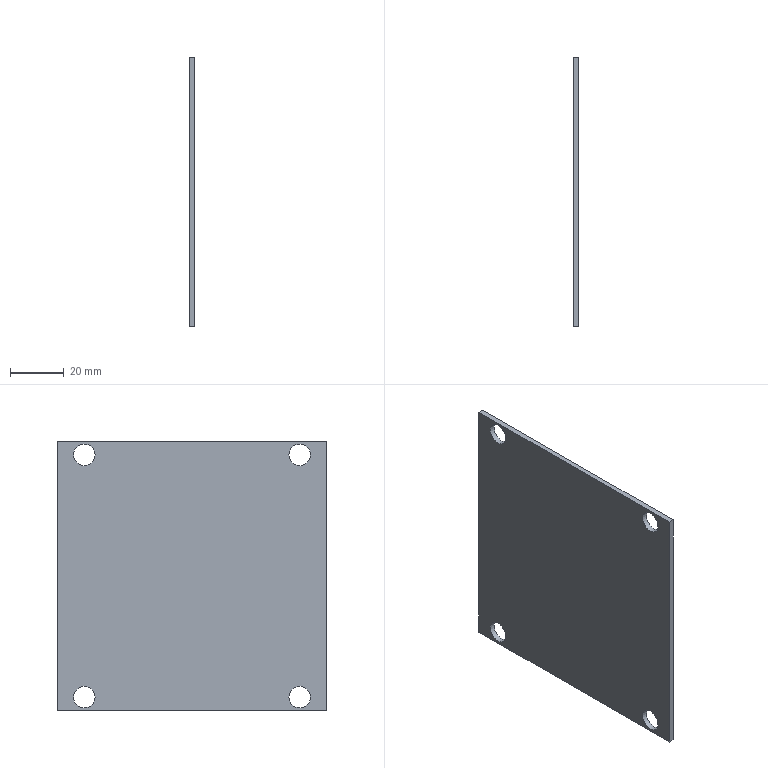Part | NX | features solid 2 | 1 solid | 10 faces | box 2 x 100 x 100 mm | volume 19598 mm3 | plane 6 | cylinder 4 | commonest cylinder face diameters 8 x4
STEP:
#1=CARTESIAN_POINT('',(1107.,-206.,-480.));
#2=VERTEX_POINT('',#1);
#3=CARTESIAN_POINT('',(1109.,-206.,-480.));
#4=VERTEX_POINT('',#3);
#5=CARTESIAN_POINT('',(1107.,-206.,-480.));
#6=DIRECTION('',(1.,0.,0.));
#7=VECTOR('',#6,1000.);
#8=LINE('',#5,#7);
#9=EDGE_CURVE('',#2,#4,#8,.T.);
#10=ORIENTED_EDGE('',*,*,#9,.F.);
#11=CARTESIAN_POINT('',(1107.,-106.,-480.));
#12=VERTEX_POINT('',#11);
#13=CARTESIAN_POINT('',(1107.,-106.,-480.));
#14=DIRECTION('',(0.,-1.,0.));
#15=VECTOR('',#14,1000.);
#16=LINE('',#13,#15);
#17=EDGE_CURVE('',#12,#2,#16,.T.);
#18=ORIENTED_EDGE('',*,*,#17,.F.);
#19=CARTESIAN_POINT('',(1109.,-106.,-480.));
#20=VERTEX_POINT('',#19);
#21=CARTESIAN_POINT('',(1107.,-106.,-480.));
#22=DIRECTION('',(1.,0.,0.));
#23=VECTOR('',#22,1000.);
#24=LINE('',#21,#23);
#25=EDGE_CURVE('',#12,#20,#24,.T.);
#26=ORIENTED_EDGE('',*,*,#25,.T.);
#27=CARTESIAN_POINT('',(1109.,-106.,-480.));
#28=DIRECTION('',(0.,1.,0.));
#29=VECTOR('',#28,1000.);
#30=LINE('',#27,#29);
#31=EDGE_CURVE('',#20,#4,#30,.F.);
#32=ORIENTED_EDGE('',*,*,#31,.T.);
#33=EDGE_LOOP('',(#10,#18,#26,#32));
#34=FACE_BOUND('',#33,.T.);
#35=CARTESIAN_POINT('',(1107.,-106.,-480.));
#36=DIRECTION('',(0.,0.,-1.));
#37=DIRECTION('',(0.,-1.,0.));
#38=AXIS2_PLACEMENT_3D('',#35,#36,#37);
#39=PLANE('',#38);
#40=ADVANCED_FACE('',(#34),#39,.T.);
#41=ORIENTED_EDGE('',*,*,#25,.F.);
#42=CARTESIAN_POINT('',(1107.,-106.,-380.));
#43=VERTEX_POINT('',#42);
#44=CARTESIAN_POINT('',(1107.,-106.,-480.));
#45=DIRECTION('',(0.,0.,1.));
#46=VECTOR('',#45,1000.);
#47=LINE('',#44,#46);
#48=EDGE_CURVE('',#12,#43,#47,.T.);
#49=ORIENTED_EDGE('',*,*,#48,.T.);
#50=CARTESIAN_POINT('',(1109.,-106.,-380.));
#51=VERTEX_POINT('',#50);
#52=CARTESIAN_POINT('',(1107.,-106.,-380.));
#53=DIRECTION('',(1.,0.,0.));
#54=VECTOR('',#53,1000.);
#55=LINE('',#52,#54);
#56=EDGE_CURVE('',#43,#51,#55,.T.);
#57=ORIENTED_EDGE('',*,*,#56,.T.);
#58=CARTESIAN_POINT('',(1109.,-106.,-480.));
#59=DIRECTION('',(0.,0.,-1.));
#60=VECTOR('',#59,1000.);
#61=LINE('',#58,#60);
#62=EDGE_CURVE('',#20,#51,#61,.F.);
#63=ORIENTED_EDGE('',*,*,#62,.F.);
#64=EDGE_LOOP('',(#41,#49,#57,#63));
#65=FACE_BOUND('',#64,.T.);
#66=CARTESIAN_POINT('',(1107.,-106.,-480.));
#67=DIRECTION('',(0.,-1.,0.));
#68=DIRECTION('',(0.,0.,1.));
#69=AXIS2_PLACEMENT_3D('',#66,#67,#68);
#70=PLANE('',#69);
#71=ADVANCED_FACE('',(#65),#70,.F.);
#72=ORIENTED_EDGE('',*,*,#56,.F.);
#73=CARTESIAN_POINT('',(1107.,-206.,-380.));
#74=VERTEX_POINT('',#73);
#75=CARTESIAN_POINT('',(1107.,-106.,-380.));
#76=DIRECTION('',(0.,-1.,0.));
#77=VECTOR('',#76,1000.);
#78=LINE('',#75,#77);
#79=EDGE_CURVE('',#43,#74,#78,.T.);
#80=ORIENTED_EDGE('',*,*,#79,.T.);
#81=CARTESIAN_POINT('',(1109.,-206.,-380.));
#82=VERTEX_POINT('',#81);
#83=CARTESIAN_POINT('',(1107.,-206.,-380.));
#84=DIRECTION('',(1.,0.,0.));
#85=VECTOR('',#84,1000.);
#86=LINE('',#83,#85);
#87=EDGE_CURVE('',#74,#82,#86,.T.);
#88=ORIENTED_EDGE('',*,*,#87,.T.);
#89=CARTESIAN_POINT('',(1109.,-106.,-380.));
#90=DIRECTION('',(0.,1.,0.));
#91=VECTOR('',#90,1000.);
#92=LINE('',#89,#91);
#93=EDGE_CURVE('',#51,#82,#92,.F.);
#94=ORIENTED_EDGE('',*,*,#93,.F.);
#95=EDGE_LOOP('',(#72,#80,#88,#94));
#96=FACE_BOUND('',#95,.T.);
#97=CARTESIAN_POINT('',(1107.,-106.,-380.));
#98=DIRECTION('',(0.,0.,-1.));
#99=DIRECTION('',(0.,-1.,0.));
#100=AXIS2_PLACEMENT_3D('',#97,#98,#99);
#101=PLANE('',#100);
#102=ADVANCED_FACE('',(#96),#101,.F.);
#103=CARTESIAN_POINT('',(1107.,-206.,-480.));
#104=DIRECTION('',(0.,0.,1.));
#105=VECTOR('',#104,1000.);
#106=LINE('',#103,#105);
#107=EDGE_CURVE('',#2,#74,#106,.T.);
#108=ORIENTED_EDGE('',*,*,#107,.F.);
#109=ORIENTED_EDGE('',*,*,#9,.T.);
#110=CARTESIAN_POINT('',(1109.,-206.,-480.));
#111=DIRECTION('',(0.,0.,-1.));
#112=VECTOR('',#111,1000.);
#113=LINE('',#110,#112);
#114=EDGE_CURVE('',#4,#82,#113,.F.);
#115=ORIENTED_EDGE('',*,*,#114,.T.);
#116=ORIENTED_EDGE('',*,*,#87,.F.);
#117=EDGE_LOOP('',(#108,#109,#115,#116));
#118=FACE_BOUND('',#117,.T.);
#119=CARTESIAN_POINT('',(1107.,-206.,-480.));
#120=DIRECTION('',(0.,-1.,0.));
#121=DIRECTION('',(0.,0.,1.));
#122=AXIS2_PLACEMENT_3D('',#119,#120,#121);
#123=PLANE('',#122);
#124=ADVANCED_FACE('',(#118),#123,.T.);
#125=CARTESIAN_POINT('',(1109.,-112.,-385.));
#126=VERTEX_POINT('',#125);
#127=CARTESIAN_POINT('',(1109.,-116.,-385.));
#128=DIRECTION('',(-1.,0.,0.));
#129=DIRECTION('',(0.,1.,0.));
#130=AXIS2_PLACEMENT_3D('',#127,#128,#129);
#131=CIRCLE('',#130,4.);
#132=EDGE_CURVE('',#126,#126,#131,.T.);
#133=ORIENTED_EDGE('',*,*,#132,.T.);
#134=EDGE_LOOP('',(#133));
#135=FACE_BOUND('',#134,.T.);
#136=CARTESIAN_POINT('',(1109.,-192.,-385.));
#137=VERTEX_POINT('',#136);
#138=CARTESIAN_POINT('',(1109.,-196.,-385.));
#139=DIRECTION('',(-1.,0.,0.));
#140=DIRECTION('',(0.,1.,0.));
#141=AXIS2_PLACEMENT_3D('',#138,#139,#140);
#142=CIRCLE('',#141,4.);
#143=EDGE_CURVE('',#137,#137,#142,.T.);
#144=ORIENTED_EDGE('',*,*,#143,.T.);
#145=EDGE_LOOP('',(#144));
#146=FACE_BOUND('',#145,.T.);
#147=CARTESIAN_POINT('',(1109.,-192.,-475.));
#148=VERTEX_POINT('',#147);
#149=CARTESIAN_POINT('',(1109.,-196.,-475.));
#150=DIRECTION('',(-1.,0.,0.));
#151=DIRECTION('',(0.,1.,0.));
#152=AXIS2_PLACEMENT_3D('',#149,#150,#151);
#153=CIRCLE('',#152,4.);
#154=EDGE_CURVE('',#148,#148,#153,.T.);
#155=ORIENTED_EDGE('',*,*,#154,.T.);
#156=EDGE_LOOP('',(#155));
#157=FACE_BOUND('',#156,.T.);
#158=CARTESIAN_POINT('',(1109.,-112.,-475.));
#159=VERTEX_POINT('',#158);
#160=CARTESIAN_POINT('',(1109.,-116.,-475.));
#161=DIRECTION('',(-1.,0.,0.));
#162=DIRECTION('',(0.,1.,0.));
#163=AXIS2_PLACEMENT_3D('',#160,#161,#162);
#164=CIRCLE('',#163,4.);
#165=EDGE_CURVE('',#159,#159,#164,.T.);
#166=ORIENTED_EDGE('',*,*,#165,.T.);
#167=EDGE_LOOP('',(#166));
#168=FACE_BOUND('',#167,.T.);
#169=ORIENTED_EDGE('',*,*,#93,.T.);
#170=ORIENTED_EDGE('',*,*,#114,.F.);
#171=ORIENTED_EDGE('',*,*,#31,.F.);
#172=ORIENTED_EDGE('',*,*,#62,.T.);
#173=EDGE_LOOP('',(#169,#170,#171,#172));
#174=FACE_BOUND('',#173,.T.);
#175=CARTESIAN_POINT('',(1109.,-106.,-480.));
#176=DIRECTION('',(-1.,0.,0.));
#177=DIRECTION('',(0.,1.,0.));
#178=AXIS2_PLACEMENT_3D('',#175,#176,#177);
#179=PLANE('',#178);
#180=ADVANCED_FACE('',(#135,#146,#157,#168,#174),#179,.F.);
#181=CARTESIAN_POINT('',(1107.,-112.,-385.));
#182=VERTEX_POINT('',#181);
#183=CARTESIAN_POINT('',(1107.,-116.,-385.));
#184=DIRECTION('',(-1.,0.,0.));
#185=DIRECTION('',(0.,1.,0.));
#186=AXIS2_PLACEMENT_3D('',#183,#184,#185);
#187=CIRCLE('',#186,4.);
#188=EDGE_CURVE('',#182,#182,#187,.T.);
#189=ORIENTED_EDGE('',*,*,#188,.F.);
#190=EDGE_LOOP('',(#189));
#191=FACE_BOUND('',#190,.T.);
#192=CARTESIAN_POINT('',(1107.,-192.,-385.));
#193=VERTEX_POINT('',#192);
#194=CARTESIAN_POINT('',(1107.,-196.,-385.));
#195=DIRECTION('',(-1.,0.,0.));
#196=DIRECTION('',(0.,1.,0.));
#197=AXIS2_PLACEMENT_3D('',#194,#195,#196);
#198=CIRCLE('',#197,4.);
#199=EDGE_CURVE('',#193,#193,#198,.T.);
#200=ORIENTED_EDGE('',*,*,#199,.F.);
#201=EDGE_LOOP('',(#200));
#202=FACE_BOUND('',#201,.T.);
#203=CARTESIAN_POINT('',(1107.,-192.,-475.));
#204=VERTEX_POINT('',#203);
#205=CARTESIAN_POINT('',(1107.,-196.,-475.));
#206=DIRECTION('',(-1.,0.,0.));
#207=DIRECTION('',(0.,1.,0.));
#208=AXIS2_PLACEMENT_3D('',#205,#206,#207);
#209=CIRCLE('',#208,4.);
#210=EDGE_CURVE('',#204,#204,#209,.T.);
#211=ORIENTED_EDGE('',*,*,#210,.F.);
#212=EDGE_LOOP('',(#211));
#213=FACE_BOUND('',#212,.T.);
#214=CARTESIAN_POINT('',(1107.,-112.,-475.));
#215=VERTEX_POINT('',#214);
#216=CARTESIAN_POINT('',(1107.,-116.,-475.));
#217=DIRECTION('',(-1.,0.,0.));
#218=DIRECTION('',(0.,1.,0.));
#219=AXIS2_PLACEMENT_3D('',#216,#217,#218);
#220=CIRCLE('',#219,4.);
#221=EDGE_CURVE('',#215,#215,#220,.T.);
#222=ORIENTED_EDGE('',*,*,#221,.F.);
#223=EDGE_LOOP('',(#222));
#224=FACE_BOUND('',#223,.T.);
#225=ORIENTED_EDGE('',*,*,#79,.F.);
#226=ORIENTED_EDGE('',*,*,#48,.F.);
#227=ORIENTED_EDGE('',*,*,#17,.T.);
#228=ORIENTED_EDGE('',*,*,#107,.T.);
#229=EDGE_LOOP('',(#225,#226,#227,#228));
#230=FACE_BOUND('',#229,.T.);
#231=CARTESIAN_POINT('',(1107.,-106.,-480.));
#232=DIRECTION('',(-1.,0.,0.));
#233=DIRECTION('',(0.,1.,0.));
#234=AXIS2_PLACEMENT_3D('',#231,#232,#233);
#235=PLANE('',#234);
#236=ADVANCED_FACE('',(#191,#202,#213,#224,#230),#235,.T.);
#237=ORIENTED_EDGE('',*,*,#221,.T.);
#238=EDGE_LOOP('',(#237));
#239=FACE_BOUND('',#238,.T.);
#240=ORIENTED_EDGE('',*,*,#165,.F.);
#241=EDGE_LOOP('',(#240));
#242=FACE_BOUND('',#241,.T.);
#243=CARTESIAN_POINT('',(1109.,-116.,-475.));
#244=DIRECTION('',(-1.,0.,0.));
#245=DIRECTION('',(0.,1.,0.));
#246=AXIS2_PLACEMENT_3D('',#243,#244,#245);
#247=CYLINDRICAL_SURFACE('',#246,4.);
#248=ADVANCED_FACE('',(#239,#242),#247,.F.);
#249=ORIENTED_EDGE('',*,*,#210,.T.);
#250=EDGE_LOOP('',(#249));
#251=FACE_BOUND('',#250,.T.);
#252=ORIENTED_EDGE('',*,*,#154,.F.);
#253=EDGE_LOOP('',(#252));
#254=FACE_BOUND('',#253,.T.);
#255=CARTESIAN_POINT('',(1109.,-196.,-475.));
#256=DIRECTION('',(-1.,0.,0.));
#257=DIRECTION('',(0.,1.,0.));
#258=AXIS2_PLACEMENT_3D('',#255,#256,#257);
#259=CYLINDRICAL_SURFACE('',#258,4.);
#260=ADVANCED_FACE('',(#251,#254),#259,.F.);
#261=ORIENTED_EDGE('',*,*,#199,.T.);
#262=EDGE_LOOP('',(#261));
#263=FACE_BOUND('',#262,.T.);
#264=ORIENTED_EDGE('',*,*,#143,.F.);
#265=EDGE_LOOP('',(#264));
#266=FACE_BOUND('',#265,.T.);
#267=CARTESIAN_POINT('',(1109.,-196.,-385.));
#268=DIRECTION('',(-1.,0.,0.));
#269=DIRECTION('',(0.,1.,0.));
#270=AXIS2_PLACEMENT_3D('',#267,#268,#269);
#271=CYLINDRICAL_SURFACE('',#270,4.);
#272=ADVANCED_FACE('',(#263,#266),#271,.F.);
#273=ORIENTED_EDGE('',*,*,#188,.T.);
#274=EDGE_LOOP('',(#273));
#275=FACE_BOUND('',#274,.T.);
#276=ORIENTED_EDGE('',*,*,#132,.F.);
#277=EDGE_LOOP('',(#276));
#278=FACE_BOUND('',#277,.T.);
#279=CARTESIAN_POINT('',(1109.,-116.,-385.));
#280=DIRECTION('',(-1.,0.,0.));
#281=DIRECTION('',(0.,1.,0.));
#282=AXIS2_PLACEMENT_3D('',#279,#280,#281);
#283=CYLINDRICAL_SURFACE('',#282,4.);
#284=ADVANCED_FACE('',(#275,#278),#283,.F.);
#285=CLOSED_SHELL('',(#40,#71,#102,#124,#180,#236,#248,#260,#272,#284));
#286=MANIFOLD_SOLID_BREP('',#285);
#287=(LENGTH_UNIT()NAMED_UNIT(*)SI_UNIT(.MILLI.,.METRE.));
#288=UNCERTAINTY_MEASURE_WITH_UNIT(LENGTH_MEASURE(0.00001),#287,'','');
#289=(NAMED_UNIT(*)PLANE_ANGLE_UNIT()SI_UNIT($,.RADIAN.));
#290=(NAMED_UNIT(*)SI_UNIT($,.STERADIAN.)SOLID_ANGLE_UNIT());
#291=(GEOMETRIC_REPRESENTATION_CONTEXT(3)GLOBAL_UNCERTAINTY_ASSIGNED_CONTEXT((#288))GLOBAL_UNIT_ASSIGNED_CONTEXT((#287,#289,#290))REPRESENTATION_CONTEXT('',''));
#292=ADVANCED_BREP_SHAPE_REPRESENTATION('',(#286),#291);